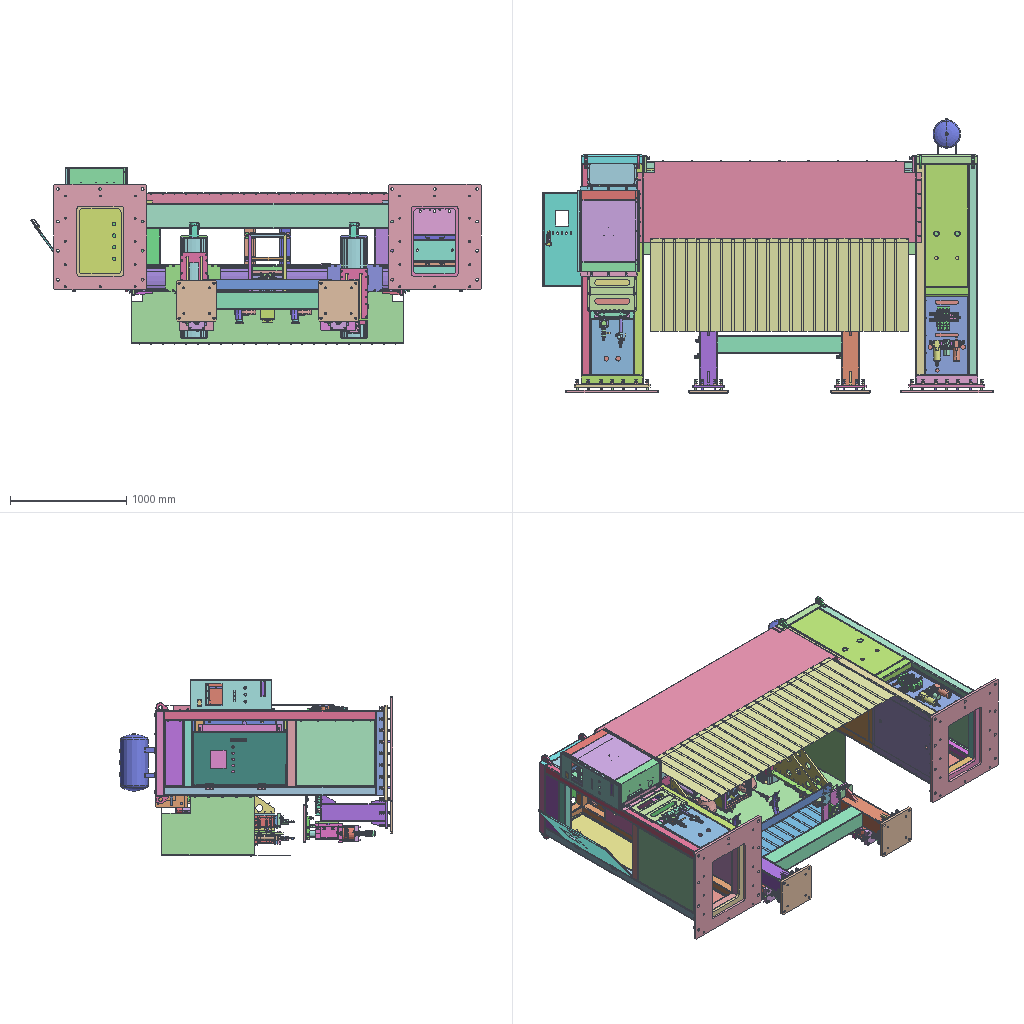Assembly | SolidWorks | 236 different items | 2045 placed | box 3873 x 2354 x 1514 mm
Parts list (item | name | quantity | parent item | size | volume | features):
1 | (subassembly) | x1 | - | - | 116635153 mm3 | -
2 | (subassembly) | x1 | in 1 | - | 39845939 mm3 | features ReferencePattern 84, LocalLPattern 9, CompositeCurve 3
3 | (subassembly) | x1 | in 1 | - | 39439593 mm3 | features ReferencePattern 3, CompositeCurve 2, LocalLPattern 1
4 | (subassembly) | x2 | in 1 | 203.047 x 914.102 x 280.36 mm | 3806317 mm3 | -
5 | (subassembly) | x2 | in 4 | 236 x 200 x 50 mm | 294173 mm3 | features HoleWzd 1
6 | (subassembly) | x2 | in 4 | 68 x 128 x 60 mm | 111810 mm3 | features HoleWzd 2
7 | (subassembly) | x1 | - | - | 32750415 mm3 | features ReferencePattern 33, LocalLPattern 4, CompositeCurve 3
8 | (subassembly) | x1 | in 26 | 248 x 227 x 99 mm | 1707610 mm3 | features AEMSimFeature 1
9 | (subassembly) | x2 | in 23 | 17.02 x 70 x 47.607 mm | 9149 mm3 | features AEMSimFeature 1
10 | (subassembly) | x1 | in 23 | 41.5 x 132 x 91.25 mm | 70272 mm3 | -
11 | (subassembly) | x2 | in 7 | 155 x 160 x 586.3 mm | 4938149 mm3 | features CompositeCurve 1
12 | (subassembly) | x2 | in 2, 3 | 305 x 58.518 x 57 mm | 304092 mm3 | features AEMSimFeature 1
13 | (subassembly) | x2 | in 14 | 152 x 98 x 38 mm | 442498 mm3 | -
14 | (subassembly) | x2 | in 7 | 152 x 98 x 38 mm | 442498 mm3 | -
15 | (subassembly) | x1 | in 25 | 91.219 x 83 x 33 mm | 40159 mm3 | -
16 | (subassembly) | x2 | in 2, 3 | 242 x 122 x 992.2 mm | 12646217 mm3 | features AEMSimFeature 1
17 | (subassembly) | x2 | in 2, 3 | 242 x 122 x 1042 mm | 13192618 mm3 | features AEMSimFeature 1
18 | (subassembly) | x2 | in 2, 3 | 35 x 30 x 30 mm | 22306 mm3 | features AEMSimFeature 1
19 | (subassembly) | x1 | in 26 | 209.8 x 130.6 x 274 mm | 1263291 mm3 | features ReferencePattern 6, LocalLPattern 1
20 | (subassembly) | x1 | in 25 | 68.642 x 53 x 59.392 mm | 27108 mm3 | -
21 | (subassembly) | x2 | in 4 | 110 x 140.16 x 248.72 mm | 144170 mm3 | -
22 | (subassembly) | x1 | in 25 | 57.569 x 74 x 99 mm | 152392 mm3 | -
23 | (subassembly) | x1 | - | - | 53716984 mm3 | features ReferencePattern 14, LocalLPattern 1
24 | (subassembly) | x1 | in 23 | 650 x 1995 x 900 mm | 30095229 mm3 | -
25 | (subassembly) | x1 | in 23 | 276.863 x 329.153 x 86.261 mm | 574652 mm3 | features CompositeCurve 2
26 | (subassembly) | x1 | - | - | 70550722 mm3 | features ReferencePattern 14, CompositeCurve 2, LocalLPattern 1
27 | (subassembly) | x1 | in 26 | 650 x 2000 x 900 mm | 28576602 mm3 | -
28 | - | x1 | in 26 | 306.443 x 240 x 500 mm | 20512353 mm3 | features ICE 5, HoleWzd 4, MirrorPattern 3, RefAxis 2, Extrusion 1, Revolution 1
29 | - | x1 | in 7 | 20.6 x 20 x 20 mm | 935.053 mm3 | features Revolution 1
30 | - | x4 | in 12 | 40 x 5.1 x 4.4 mm | 573.817 mm3 | features BaseBody 1
31 | - | x6 | in 16 | 13 x 15.5 x 39.5 mm | 3396 mm3 | features ICE 19, HoleWzd 5, Extrusion 1
32 | - | x6 | in 17 | 13 x 15.5 x 39.5 mm | 3396 mm3 | features ICE 19, HoleWzd 5, Extrusion 1
33 | - | x2 | in 16 | 220 x 113.5 x 15 mm | 261073 mm3 | features ICE 4, Chamfer 3, Extrusion 1, Fillet 1, HoleWzd 1
34 | - | x2 | in 17 | 220 x 113.5 x 15 mm | 261073 mm3 | features ICE 4, Chamfer 3, Extrusion 1, Fillet 1, HoleWzd 1
35 | - | x2 | in 16 | 188.037 x 25 x 1150 mm | 3794355 mm3 | features Extrusion 1, Fillet 1
36 | - | x2 | in 17 | 188.037 x 25 x 900 mm | 2969495 mm3 | features Extrusion 1, Fillet 1
37 | - | x2 | in 16 | 220 x 113.5 x 5 mm | 112175 mm3 | features Fillet 2, ICE 2, Chamfer 1, Extrusion 1
38 | - | x2 | in 17 | 220 x 113.5 x 5 mm | 112175 mm3 | features Fillet 2, ICE 2, Chamfer 1, Extrusion 1
39 | - | x2 | in 16 | 7 x 26.5 x 18 mm | 793.289 mm3 | features CornerTrim 1, FlatPattern 1, ICE 1, SMBaseFlange 1, SheetMetal 1
40 | - | x2 | in 16 | 220 x 67.5 x 1150 mm | 8709767 mm3 | features HoleWzd 3, ICE 3, Extrusion 1, Fillet 1, LPattern 1
41 | - | x2 | in 17 | 220 x 67.5 x 900 mm | 6810369 mm3 | features HoleWzd 3, ICE 3, Extrusion 1, Fillet 1, LPattern 1
42 | - | x2 | in 16 | 230 x 60 x 480 mm | 2333342 mm3 | features ICE 9, Fillet 3, HoleWzd 2, Chamfer 1, Cut 1, Extrusion 1, MirrorPattern 1
43 | - | x2 | in 17 | 230 x 60 x 480 mm | 2333342 mm3 | features ICE 9, Fillet 3, HoleWzd 2, Chamfer 1, Cut 1, Extrusion 1, MirrorPattern 1
44 | - | x2 | in 26 | 43.5 x 46 x 54 mm | 41092 mm3 | features BaseBody 1
45 | - | x4 | in 12 | 18 x 12.6 x 23 mm | 2035 mm3 | features BaseBody 1
46 | - | x4 | in 12 | 38 x 21 x 57 mm | 7816 mm3 | features BaseBody 1
47 | - | x2 | in 8 | 76 x 79.5 x 15.5 mm | 53255 mm3 | features BaseBody 1
48 | - | x1 | in 8 | 80 x 202.5 x 68 mm | 579205 mm3 | features BaseBody 1
49 | - | x1 | in 8 | 80 x 204.5 x 68 mm | 577118 mm3 | features BaseBody 1
50 | - | x2 | in 17 | 7 x 26.5 x 18 mm | 793.289 mm3 | features CornerTrim 1, FlatPattern 1, ICE 1, SMBaseFlange 1, SheetMetal 1
51 | - | x1 | in 8 | 80 x 140.5 x 83 mm | 444792 mm3 | features BaseBody 1
52 | - | x4 | in 7 | 70 x 25 x 14 mm | 23519 mm3 | features Extrusion 1, Fillet 1
53 | - | x2 | in 2 | 10 x 10 x 24 mm | 1497 mm3 | features Chamfer 3, Cut 2, Extrusion 1, RevCut 1
54 | - | x4 | - | 16 x 16 x 32 mm | 5349 mm3 | features Chamfer 3, Cut 2, Extrusion 1, RevCut 1
55 | - | x4 | in 2 | 6 x 6 x 22 mm | 513.442 mm3 | features Chamfer 3, Cut 2, Extrusion 1, RevCut 1
56 | - | x4 | in 2 | 8 x 8 x 30 mm | 1303 mm3 | features Chamfer 3, Cut 2, Extrusion 1, RevCut 1
57 | - | x78 | in 7, 23, 26 | 26.17 x 22.664 x 15.9 mm | 3864 mm3 | features Cut 2, Chamfer 1, Extrusion 1
58 | - | x4 | in 2 | 55.3 x 15.011 x 13 mm | 3268 mm3 | features RevCut 4, Chamfer 1, Extrusion 1, Fillet 1, LPattern 1, Revolution 1
59 | - | x4 | in 7 | 30.3 x 15.011 x 13 mm | 2011 mm3 | features RevCut 4, Chamfer 1, Extrusion 1, Fillet 1, LPattern 1, Revolution 1
60 | - | x50 | in 19 | 6.649 x 7.66 x 3.2 mm | 79.578 mm3 | features Cut 2, Chamfer 1, Extrusion 1
61 | - | x2 | in 25 | 26 x 31 x 10 mm | 2120 mm3 | features ICE 2, Revolution 1, Sweep 1
62 | - | x2 | in 26 | 12.482 x 14.38 x 6.8 mm | 562.42 mm3 | features Cut 2, Chamfer 1, Extrusion 1
63 | - | x4 | in 7 | 12.482 x 14.38 x 4 mm | 327.094 mm3 | features Cut 2, Chamfer 1, Extrusion 1
64 | - | x4 | in 2 | 30 x 16 x 16 mm | 3296 mm3 | features BlendCut 1, Cut 1, Fillet 1, LPattern 1, RevCut 1, Revolution 1
65 | - | x16 | in 4, 7 | 40 x 16 x 16 mm | 4081 mm3 | features BlendCut 1, Cut 1, Fillet 1, LPattern 1, RevCut 1, Revolution 1
66 | - | x6 | in 2 | 45 x 16 x 16 mm | 4474 mm3 | features BlendCut 1, Cut 1, Fillet 1, LPattern 1, RevCut 1, Revolution 1
67 | - | x32 | in 7, 23, 26 | 116 x 24 x 24 mm | 25974 mm3 | features BlendCut 1, Cut 1, Fillet 1, LPattern 1, RevCut 1, Revolution 1
68 | - | x20 | - | 56 x 24 x 24 mm | 13910 mm3 | features BlendCut 1, Cut 1, Fillet 1, LPattern 1, RevCut 1, Revolution 1
69 | - | x12 | in 7 | 71 x 24 x 24 mm | 16926 mm3 | features BlendCut 1, Cut 1, Fillet 1, LPattern 1, RevCut 1, Revolution 1
70 | - | x44 | in 7, 23, 26 | 96 x 24 x 24 mm | 21953 mm3 | features BlendCut 1, Cut 1, Fillet 1, LPattern 1, RevCut 1, Revolution 1
71 | - | x28 | in 16 | 9 x 5.5 x 5.5 mm | 106.317 mm3 | features BlendCut 1, Cut 1, Fillet 1, RevCut 1, Revolution 1
72 | - | x8 | in 2, 25 | 16.166 x 31 x 14 mm | 2228 mm3 | features ICE 3, Chamfer 1, Revolution 1
73 | - | x28 | in 17 | 9 x 5.5 x 5.5 mm | 106.317 mm3 | features BlendCut 1, Cut 1, Fillet 1, RevCut 1, Revolution 1
74 | - | x46 | - | 16 x 7 x 7 mm | 288.227 mm3 | features BlendCut 1, Cut 1, Fillet 1, LPattern 1, RevCut 1, Revolution 1
75 | - | x4 | in 19 | 44 x 7 x 7 mm | 640.086 mm3 | features BlendCut 1, Cut 1, Fillet 1, LPattern 1, RevCut 1, Revolution 1
76 | - | x222 | in 23, 26 | 12 x 7 x 7 mm | 237.962 mm3 | features BlendCut 1, Cut 1, Fillet 1, LPattern 1, RevCut 1, Revolution 1
77 | - | x38 | - | 16 x 10 x 10 mm | 686.638 mm3 | features BlendCut 1, Cut 1, Fillet 1, LPattern 1, RevCut 1, Revolution 1
78 | - | x8 | in 7 | 26 x 10 x 10 mm | 969.381 mm3 | features BlendCut 1, Cut 1, Fillet 1, LPattern 1, RevCut 1, Revolution 1
79 | - | x4 | in 7 | 36 x 10 x 10 mm | 1252 mm3 | features BlendCut 1, Cut 1, Fillet 1, LPattern 1, RevCut 1, Revolution 1
80 | - | x4 | in 7 | 46 x 10 x 10 mm | 1535 mm3 | features BlendCut 1, Cut 1, Fillet 1, LPattern 1, RevCut 1, Revolution 1
81 | - | x10 | in 23 | 24 x 13 x 13 mm | 1736 mm3 | features BlendCut 1, Cut 1, Fillet 1, LPattern 1, RevCut 1, Revolution 1
82 | - | x28 | in 7 | 28 x 13 x 13 mm | 1937 mm3 | features BlendCut 1, Cut 1, Fillet 1, LPattern 1, RevCut 1, Revolution 1
83 | - | x1 | in 19 | 75 x 28 x 192 mm | 234020 mm3 | features BaseBody 1
84 | - | x49 | in 2, 26 | 33 x 13 x 13 mm | 2189 mm3 | features BlendCut 1, Cut 1, Fillet 1, LPattern 1, RevCut 1, Revolution 1
85 | - | x28 | in 2 | 38 x 13 x 13 mm | 2440 mm3 | features BlendCut 1, Cut 1, Fillet 1, LPattern 1, RevCut 1, Revolution 1
86 | - | x28 | in 2, 23 | 48 x 13 x 13 mm | 2943 mm3 | features BlendCut 1, Cut 1, Fillet 1, LPattern 1, RevCut 1, Revolution 1
87 | - | x12 | in 23 | 10 x 8.96 x 8.96 mm | 171.604 mm3 | features RevCut 2, Revolution 2, Cut 1, LPattern 1, RefAxis 1
88 | - | x4 | in 4 | 10 x 8 x 8 mm | 368.793 mm3 | features RevCut 2, Cut 1, LPattern 1, Revolution 1
89 | - | x18 | in 2, 4 | 15.372 x 15.344 x 2.6 mm | 261.313 mm3 | features Extrusion 1
90 | - | x32 | in 7 | 24.356 x 24.313 x 4.1 mm | 1031 mm3 | features Extrusion 1
91 | - | x272 | in 19, 23, 26 | 6.287 x 6.275 x 1.1 mm | 18.963 mm3 | features Extrusion 1
92 | - | x46 | in 7 | 9.282 x 9.265 x 1.6 mm | 59.463 mm3 | features Extrusion 1
93 | - | x30 | in 2, 23 | 12.277 x 12.254 x 2.1 mm | 135.755 mm3 | features Extrusion 1
94 | - | x4 | in 19 | 27 x 69.3 x 209.8 mm | 222441 mm3 | features BaseBody 1
95 | - | x8 | in 4 | 20 x 2 x 20 mm | 438.252 mm3 | features Revolution 1
96 | - | x32 | in 7 | 30 x 3 x 30 mm | 1399 mm3 | features Revolution 1
97 | - | x276 | in 19, 23, 26 | 9 x 0.8 x 9 mm | 38.17 mm3 | features Revolution 1
98 | - | x46 | in 7 | 12 x 1.6 x 12 mm | 127.863 mm3 | features Revolution 1
99 | - | x26 | in 23 | 16 x 1.6 x 16 mm | 219.911 mm3 | features Revolution 1
100 | - | x4 | in 2 | 20 x 2 x 20 mm | 455.138 mm3 | features Revolution 1
101 | - | x2 | in 9 | 8 x 70 x 29 mm | 3838 mm3 | features BaseBody 1
102 | - | x2 | in 9 | 8 x 70 x 29 mm | 4432 mm3 | features BaseBody 1
103 | - | x2 | in 9 | 4 x 70 x 4 mm | 879.661 mm3 | features BaseBody 1
104 | - | x1 | in 23 | - | 3525284 mm3 | features BaseBody 46
105 | - | x1 | in 25 | 33.486 x 29 x 29 mm | 7069 mm3 | features ICE 3, Chamfer 1, Extrusion 1, HoleWzd 1
106 | - | x1 | in 1 | 128 x 196 x 428.2 mm | 1860120 mm3 | features BaseBody 23
107 | - | x2 | in 19 | 64.8 x 11 x 27.5 mm | 5589 mm3 | features BaseBody 1
108 | - | x2 | in 19 | 26 x 68 x 26.213 mm | 26023 mm3 | features BaseBody 1
109 | - | x1 | in 26 | 19.63 x 32.5 x 17 mm | 4456 mm3 | features BaseBody 1
110 | - | x2 | in 19 | 35.315 x 37 x 18 mm | 6710 mm3 | features BaseBody 1
111 | - | x2 | in 26 | 37.624 x 41.5 x 21 mm | 10136 mm3 | features BaseBody 1
112 | - | x3 | in 19 | 32.815 x 34 x 17 mm | 6015 mm3 | features BaseBody 1
113 | - | x1 | in 19 | 35.315 x 63.5 x 18 mm | 9000 mm3 | features BaseBody 1
114 | - | x3 | in 19 | 32.815 x 55.5 x 17 mm | 7231 mm3 | features BaseBody 1
115 | - | x4 | in 7 | 49.5 x 58.5 x 28 mm | 24100 mm3 | features BaseBody 1
116 | - | x2 | in 11 | 125 x 125 x 5.7 mm | 25182 mm3 | features BaseBody 1
117 | - | x4 | in 7 | 33.5 x 41.5 x 15 mm | 5375 mm3 | features BaseBody 1
118 | - | x2 | in 2 | 37.5 x 47.5 x 18 mm | 8206 mm3 | features BaseBody 1
119 | - | x4 | in 2 | 40.75 x 52.5 x 22.5 mm | 13948 mm3 | features BaseBody 1
120 | - | x8 | in 12 | 22 x 10 x 10 mm | 853.724 mm3 | features BaseBody 1
121 | - | x2 | in 12 | 7 x 19.63 x 17 mm | 1102 mm3 | features BaseBody 1
122 | - | x2 | in 12 | 232.5 x 39.5 x 39.5 mm | 68995 mm3 | features BaseBody 1
123 | - | x2 | in 12 | 233 x 50 x 50 mm | 209735 mm3 | features BaseBody 1
124 | - | x2 | in 13 | 136 x 38 x 98 mm | 311223 mm3 | features BaseBody 1
125 | - | x2 | in 13 | 143.5 x 36 x 96 mm | 131275 mm3 | features BaseBody 1
126 | - | x2 | in 11 | 25 x 25 x 150 mm | 71513 mm3 | features BaseBody 1
127 | - | x6 | in 16 | 25 x 17 x 16 mm | 1093 mm3 | features EdgeFlange 1, Fillet 1, FlatPattern 1, HoleWzd 1, ICE 1, MirrorPattern 1, SMBaseFlange 1, SheetMetal 1
128 | - | x8 | in 11 | 14.038 x 16 x 170 mm | 19424 mm3 | features BaseBody 1
129 | - | x2 | in 11 | 229 x 32 x 32 mm | 152492 mm3 | features BaseBody 1
130 | - | x2 | in 11 | 50 x 50 x 5 mm | 5541 mm3 | features BaseBody 1
131 | - | x2 | in 11 | 44.103 x 44.731 x 12 mm | 9622 mm3 | features BaseBody 1
132 | - | x2 | in 16 | 80.44 x 89.02 x 162.2 mm | 690477 mm3 | features BaseBody 1
133 | - | x2 | in 17 | 80.44 x 89.02 x 162.2 mm | 690477 mm3 | features BaseBody 1
134 | - | x2 | in 21 | 94 x 8 x 103 mm | 10565 mm3 | features ICE 1, Sweep 1
135 | - | x4 | in 21 | 15.011 x 13 x 7.9 mm | 844.03 mm3 | features Chamfer 2, RevCut 2, Extrusion 1, ICE 1, LPattern 1
136 | - | x4 | in 21 | 15.011 x 13 x 4 mm | 430.713 mm3 | features RevCut 2, Chamfer 1, Extrusion 1, LPattern 1
137 | - | x2 | in 4 | 20 x 15.24 x 15.24 mm | 1317 mm3 | features RevCut 3, Chamfer 1, Cut 1, Fillet 1, LPattern 1, Revolution 1
138 | - | x2 | in 18 | 28 x 30 x 30 mm | 9162 mm3 | features BaseBody 1
139 | - | x6 | in 17 | 25 x 17 x 16 mm | 1093 mm3 | features EdgeFlange 1, Fillet 1, FlatPattern 1, HoleWzd 1, ICE 1, MirrorPattern 1, SMBaseFlange 1, SheetMetal 1
140 | - | x1 | in 27 | 650 x 2000 x 880 mm | 28196687 mm3 | features HoleWzd 24, WeldCornerFeat 14, ICE 8, WeldMemberFeat 4, Chamfer 2, Fillet 2, 3DProfileFeature 1, WeldmentFeature 1
141 | - | x4 | in 24 | 70 x 110 x 20 mm | 94979 mm3 | features Fillet 3, Extrusion 1, ICE 1
142 | - | x4 | in 27 | 70 x 110 x 20 mm | 94979 mm3 | features Fillet 3, Extrusion 1, ICE 1
143 | - | x1 | in 24 | 650 x 1995 x 880 mm | 29715314 mm3 | features HoleWzd 25, WeldCornerFeat 15, ICE 11, Chamfer 8, WeldMemberFeat 3, Fillet 2, LPattern 2, MoveFace 2, 3DProfileFeature 1, WeldmentFeature 1
144 | - | x4 | in 21 | 16 x 16 x 1.6 mm | 233.031 mm3 | features Extrusion 1
145 | - | x2 | in 4 | 130 x 538 x 180 mm | 2549222 mm3 | features BaseBody 3
146 | - | x1 | in 25 | 27 x 27 x 154 mm | 47629 mm3 | features ICE 2, Chamfer 1, Extrusion 1, MirrorPattern 1
147 | - | x1 | in 25 | 240 x 40 x 30 mm | 239495 mm3 | features HoleWzd 6, MirrorPattern 2, Extrusion 1
148 | - | x2 | in 25 | 31.177 x 58 x 27 mm | 12376 mm3 | features ICE 4, Chamfer 2, Revolution 1
149 | - | x2 | in 11 | 125 x 125 x 8.6 mm | 37994 mm3 | features BaseBody 1
150 | - | x2 | in 2, 3 | 100 x 577.1 x 113 mm | 2394119 mm3 | features BaseBody 23, ICE 1
151 | - | x2 | in 21 | 110 x 51.16 x 248.72 mm | 85285 mm3 | features Chamfer 4, Fillet 2, HoleWzd 2, ICE 2, BossThin 1, Revolution 1, Shell 1
152 | - | x2 | in 21 | 110 x 15 x 125 mm | 45305 mm3 | features Chamfer 4, Fillet 2, ICE 2, ExtruThin 1, HoleWzd 1
153 | - | x3 | in 19 | 19.63 x 16 x 17 mm | 3623 mm3 | features BaseBody 1
154 | - | x1 | in 22 | 41.569 x 55 x 99 mm | 62530 mm3 | features ICE 5, HoleWzd 2, Extrusion 1, MirrorPattern 1
155 | - | x2 | in 22 | 74 x 74 x 13 mm | 39480 mm3 | features ICE 2, 3DProfileFeature 1, Chamfer 1, Extrusion 1, HoleWzd 1
156 | - | x1 | in 22 | 54.5 x 54.5 x 4 mm | 9331 mm3 | features Extrusion 1
157 | - | x2 | in 11 | 130 x 130 x 30 mm | 407669 mm3 | features BaseBody 1
158 | - | x1 | in 22 | 55 x 55 x 2 mm | 1571 mm3 | features Extrusion 1
159 | - | x1 | in 25 | 31.177 x 27 x 27 mm | 5569 mm3 | features ICE 3, Extrusion 1, SweepThread 1
160 | - | x1 | in 25 | 31.177 x 27 x 43 mm | 12851 mm3 | features ICE 2, Chamfer 1, Extrusion 1, MirrorPattern 1
161 | - | x1 | in 15 | 30 x 30 x 15.2 mm | 4101 mm3 | features ICE 3, Extrusion 1
162 | - | x1 | in 20 | 33 x 53.25 x 53 mm | 25680 mm3 | features ICE 10, HoleWzd 2, 3DProfileFeature 1, Extrusion 1, Fillet 1
163 | - | x1 | in 15 | 33 x 81.096 x 83 mm | 34631 mm3 | features ICE 13, HoleWzd 3, 3DProfileFeature 2, Extrusion 1, Fillet 1, Sweep 1
164 | - | x2 | in 15, 20 | 62.879 x 15.737 x 21.142 mm | 1428 mm3 | features EdgeFlange 4, Fillet 2, ICE 2, FlatPattern 1, SMBaseFlange 1, SheetMetal 1
165 | - | x2 | in 7 | 140 x 25 x 36 mm | 123238 mm3 | features Chamfer 1, Extrusion 1, HoleWzd 1
166 | - | x1 | - | 2461 x 800 x 510 mm | 7657970 mm3 | features ICE 4, EdgeFlange 2, LPattern 2, FlatPattern 1, SMBaseFlange 1, SheetMetal 1
167 | - | x1 | - | 2441 x 700 x 150 mm | 4096211 mm3 | features ICE 4, EdgeFlange 3, LPattern 2, FlatPattern 1, SMBaseFlange 1, SheetMetal 1
168 | - | x2 | in 11 | 160 x 155 x 246 mm | 1955692 mm3 | features ICE 2, BaseBody 1
169 | - | x22 | - | 120 x 350 x 2 mm | 83936 mm3 | features Extrusion 1, ICE 1
170 | - | x22 | - | 120 x 800 x 2 mm | 191936 mm3 | features Extrusion 1, ICE 1
171 | - | x1 | in 23 | 420 x 180 x 2 mm | 150541 mm3 | features RefAxis 2, Extrusion 1, Fillet 1, HoleWzd 1, ICE 1
172 | - | x2 | in 23, 26 | 1048 x 368 x 25 mm | 891323 mm3 | features EdgeFlange 1, FlatPattern 1, ICE 1, SMBaseFlange 1, SheetMetal 1
173 | - | x2 | in 23, 26 | 568 x 158 x 25 mm | 241019 mm3 | features EdgeFlange 1, FlatPattern 1, ICE 1, SMBaseFlange 1, SheetMetal 1
174 | - | x2 | in 23, 26 | 680 x 568 x 25 mm | 878615 mm3 | features EdgeFlange 1, FlatPattern 1, ICE 1, SMBaseFlange 1, SheetMetal 1
175 | - | x2 | in 23, 26 | 680 x 368 x 25 mm | 589246 mm3 | features EdgeFlange 1, FlatPattern 1, ICE 1, SMBaseFlange 1, SheetMetal 1
176 | - | x1 | in 23 | 700 x 780 x 2 mm | 1090782 mm3 | features Extrusion 1, ICE 1
177 | - | x1 | in 23 | 420 x 300 x 2 mm | 193243 mm3 | features ICE 2, Extrusion 1, Fillet 1, HoleWzd 1, MirrorPattern 1
178 | - | x1 | in 23 | 500 x 714 x 50 mm | 1369290 mm3 | features EdgeFlange 2, FlatPattern 1, ICE 1, SMBaseFlange 1, SheetMetal 1
179 | - | x2 | in 11 | 24 x 124 x 124 mm | 184707 mm3 | features BaseBody 1
180 | - | x1 | in 23 | 566 x 15 x 806 mm | 720879 mm3 | features ICE 3, EdgeFlange 2, Cut 1, FlatPattern 1, LPattern 1, SMBaseFlange 1, SheetMetal 1
181 | - | x2 | in 23 | 47 x 25 x 20 mm | 4405 mm3 | features EdgeFlange 2, Fillet 1, FlatPattern 1, ICE 1, SMBaseFlange 1, SheetMetal 1
182 | - | x1 | in 23 | 40 x 35 x 50 mm | 8331 mm3 | features EdgeFlange 3, RefAxis 3, Fillet 2, ICE 2, FlatPattern 1, SMBaseFlange 1, SheetMetal 1
183 | - | x1 | in 23 | 700 x 500 x 2 mm | 691794 mm3 | features Extrusion 1, HoleWzd 1, ICE 1
184 | - | x2 | in 23, 26 | 800 x 905 x 20 mm | 9564492 mm3 | features HoleWzd 2, ICE 2, Chamfer 1, Extrusion 1, Fillet 1
185 | - | x1 | in 23 | 479 x 368 x 25 mm | 418826 mm3 | features ICE 2, EdgeFlange 1, FlatPattern 1, SMBaseFlange 1, SheetMetal 1
186 | - | x1 | in 23 | 15 x 650 x 420 mm | 545219 mm3 | features ICE 4, EdgeFlange 1, FlatPattern 1, HoleWzd 1, SMBaseFlange 1, SheetMetal 1
187 | - | x1 | in 23 | 700 x 900 x 2 mm | 1238676 mm3 | features ICE 2, Extrusion 1
188 | - | x1 | in 26 | 810 x 570 x 25 mm | 1040756 mm3 | features EdgeFlange 1, FlatPattern 1, ICE 1, SMBaseFlange 1, SheetMetal 1
189 | - | x1 | in 26 | 680 x 370 x 25 mm | 562100 mm3 | features ICE 4, Cut 1, EdgeFlange 1, FlatPattern 1, HoleWzd 1, SMBaseFlange 1, SheetMetal 1
190 | - | x2 | in 11 | 135 x 135 x 104.3 mm | 212984 mm3 | features BaseBody 1
191 | - | x1 | in 26 | 1050 x 370 x 25 mm | 888515 mm3 | features ICE 2, Cut 1, EdgeFlange 1, FlatPattern 1, LPattern 1, SMBaseFlange 1, SheetMetal 1
192 | - | x1 | in 26 | 295 x 500 x 2 mm | 292699 mm3 | features Extrusion 1, HoleWzd 1, ICE 1
193 | - | x1 | in 26 | 355 x 500 x 2 mm | 307692 mm3 | features ICE 2, Extrusion 1, Fillet 1, HoleWzd 1
194 | - | x1 | in 26 | 700 x 900 x 2 mm | 1258782 mm3 | features Extrusion 1, ICE 1
195 | - | x1 | in 26 | 700 x 760 x 2 mm | 1059954 mm3 | features Cut 1, Extrusion 1, ICE 1
196 | - | x1 | in 1 | 2320 x 250 x 830 mm | 26047489 mm3 | features ICE 14, HoleWzd 6, WeldMemberFeat 3, Chamfer 2, 3DProfileFeature 1, Cut 1, WeldCornerFeat 1, WeldmentFeature 1
197 | - | x1 | in 1 | 523 x 375 x 640 mm | 1667392 mm3 | features WeldCornerFeat 4, HoleWzd 2, ICE 2, 3DProfileFeature 1, WeldMemberFeat 1, WeldmentFeature 1
198 | - | x2 | in 1 | 260 x 45 x 50 mm | 79882 mm3 | features ICE 2, Chamfer 1, FlatPattern 1, SMBaseFlange 1, SheetMetal 1
199 | - | x1 | in 2 | 480 x 880 x 16 mm | 3786407 mm3 | features HoleWzd 4, Chamfer 1, Extrusion 1, Fillet 1, ICE 1
200 | - | x2 | in 2, 3 | 480 x 235 x 16 mm | 1317910 mm3 | features HoleWzd 5, ICE 3, Chamfer 1, Extrusion 1, Fillet 1, LPattern 1
201 | - | x2 | in 11 | 50 x 50 x 75 mm | 76101 mm3 | features BaseBody 1
202 | - | x1 | in 2 | 16 x 550 x 235 mm | 1648146 mm3 | features HoleWzd 5, ICE 4, Chamfer 1, Extrusion 1, Fillet 1, LPattern 1
203 | - | x4 | in 2, 3 | 385 x 550 x 16 mm | 1761626 mm3 | features HoleWzd 2, LPattern 2, Extrusion 1, ICE 1
204 | - | x2 | in 2, 3 | 100 x 80 x 2 mm | 14938 mm3 | features Extrusion 1, ICE 1
205 | - | x1 | in 2 | 120 x 80 x 95 mm | 309106 mm3 | features HoleWzd 5, ICE 4, Chamfer 1, Extrusion 1, Fillet 1, RevCut 1
206 | - | x2 | in 2, 3 | 50 x 18 x 18 mm | 5917 mm3 | features ICE 1, Revolution 1
207 | - | x2 | in 2, 3 | 16 x 25 x 16 mm | 2776 mm3 | features Chamfer 1, Extrusion 1, RevCut 1
208 | - | x2 | in 2, 3 | 60 x 345 x 16 mm | 288953 mm3 | features RefAxis 4, HoleWzd 3, ICE 2, Chamfer 1, Extrusion 1
209 | - | x8 | in 2, 3 | 12.4 x 18 x 18 mm | 530.163 mm3 | features Revolution 1
210 | - | x1 | in 3 | 480 x 880 x 16 mm | 3786407 mm3 | features HoleWzd 4, Chamfer 2, Extrusion 1, Fillet 1, ICE 1
211 | - | x1 | in 3 | 16 x 550 x 235 mm | 1648646 mm3 | features HoleWzd 5, ICE 4, Chamfer 1, Extrusion 1, Fillet 1, LPattern 1
212 | - | x2 | in 11 | 145 x 145 x 40 mm | 721249 mm3 | features BaseBody 1, Cut 1
213 | - | x1 | in 3 | 110 x 80 x 95 mm | 289106 mm3 | features HoleWzd 5, ICE 4, Chamfer 1, Extrusion 1, Fillet 1, RevCut 1
214 | - | x2 | in 5 | 50 x 50 x 200 mm | 131874 mm3 | features Extrusion 1, ICE 1, WeldmentFeature 1
215 | - | x2 | in 5 | 20 x 120 x 5 mm | 9312 mm3 | features Chamfer 1, Extrusion 1
216 | - | x2 | in 5 | 50 x 50 x 200 mm | 141372 mm3 | features Extrusion 1
217 | - | x2 | in 5 | 50 x 50 x 6 mm | 11781 mm3 | features Extrusion 1
218 | - | x2 | in 4 | 100 x 100 x 366 mm | 643224 mm3 | features ICE 3, HoleWzd 2, Chamfer 1, Extrusion 1
219 | - | x2 | in 6 | 68 x 68 x 60 mm | 90478 mm3 | features Extrusion 1, WeldmentFeature 1
220 | - | x2 | in 6 | 60 x 60 x 10 mm | 21914 mm3 | features Chamfer 2, Extrusion 1
221 | - | x2 | in 4 | 50 x 50 x 5 mm | 9077 mm3 | features Chamfer 1, Extrusion 1, HoleWzd 1
222 | - | x2 | in 4 | 50 x 50 x 5 mm | 3534 mm3 | features Extrusion 1
223 | - | x2 | in 11 | 379.7 x 60 x 60 mm | 998065 mm3 | features BaseBody 1
224 | - | x2 | in 4 | 70 x 70 x 8 mm | 29565 mm3 | features Chamfer 1, Extrusion 1, HoleWzd 1
225 | - | x1 | in 7 | 1490 x 295 x 618 mm | 10128705 mm3 | features ICE 6, HoleWzd 5, Chamfer 4, 3DProfileFeature 1, MirrorPattern 1, WeldMemberFeat 1, WeldmentFeature 1
226 | - | x1 | in 7 | 1100 x 80 x 10 mm | 856189 mm3 | features ICE 2, Extrusion 1, HoleWzd 1
227 | - | x2 | in 7 | 130 x 130 x 4 mm | 65444 mm3 | features Chamfer 1, Extrusion 1, HoleWzd 1
228 | - | x1 | in 7 | 300 x 320 x 20 mm | 1873413 mm3 | features HoleWzd 2, Chamfer 1, Extrusion 1, ICE 1
229 | - | x2 | in 7 | 350 x 350 x 20 mm | 2411003 mm3 | features HoleWzd 2, Chamfer 1, Extrusion 1
230 | - | x2 | in 7 | 180 x 45 x 20 mm | 111535 mm3 | features HoleWzd 2, Chamfer 1, Extrusion 1, Fillet 1, ICE 1
231 | - | x2 | in 7 | 180 x 45 x 20 mm | 111535 mm3 | features HoleWzd 2, Chamfer 1, Extrusion 1, Fillet 1, ICE 1
232 | - | x1 | in 7 | 300 x 320 x 20 mm | 1873413 mm3 | features HoleWzd 2, Chamfer 1, Extrusion 1, ICE 1
233 | - | x2 | in 7 | 200 x 90 x 10 mm | 176073 mm3 | features HoleWzd 2, ICE 2, Extrusion 1
234 | - | x2 | in 18 | 25 x 30 x 30 mm | 13143 mm3 | features BaseBody 1
235 | SR20008JN (subassembly) | x1 | - | - | - | -
236 | Nameplate | x1 | - | - | - | -
Mates (type | each side: item.copy, entity, surface, feature), first 379 of 3009 lines:
In the top assembly
Coincident | 23.1 plane | assembly plane | 3 times
Coincident | 23.1 plane | 26.1 plane
Coincident | 143.1 face plane Cut-Extrude 2 | 196.1 face plane Boss-Extrude 4 | 2 times
Coincident | 140.1 face plane Cut-Extrude 2 | 196.1 face plane Boss-Extrude 1 | 2 times
Coincident | 184.1 face plane Boss-Extrude 1 | 229.1 face plane Boss-Extrude 1
Width | 168.1 face plane Import 1 | 168.2 face plane Import 1 | 196.1 face plane Boss-Extrude 1 | 196.1 face plane Boss-Extrude 4
DistanceDim | 225.1 face plane Boss-Extrude 8 | 140.1 face plane Square Tube 80×80×4.0(2)
Coincident | 140.1 face plane Square Tube 80×80×4.0(2) | 166.1 face plane Edge-Flange 2
Coincident | 196.1 face plane Rect Tube 220×140×5(1) | 166.1 face plane Edge-Flange 1
Width | 166.1 face plane Edge-Flange 1 | 166.1 face plane Edge-Flange 1 | 196.1 face plane Boss-Extrude 1 | 196.1 face plane Boss-Extrude 4
Width | 167.1 face plane Edge-Flange 1 | 167.1 face plane Edge-Flange 1 | 196.1 face plane Boss-Extrude 4 | 196.1 face plane Boss-Extrude 1
Coincident | 143.1 face plane Square Tube 80×80×4.0(2) | 167.1 face plane Edge-Flange 2
Coincident | 196.1 face plane Rect Tube 220×140×5(1) | 167.1 face plane Edge-Flange 3
Coincident | 166.1 face plane Base-Flange 1 | 169.1 face plane Boss-Extrude 1
Concentric | 166.1 face cylinder Cut-Extrude 6 | 169.1 face cylinder Cut-Extrude 1
Concentric | 166.1 face cylinder LPattern 2 | 169.1 face cylinder Cut-Extrude 1
Coincident | 167.1 face plane Base-Flange 1 | 170.1 face plane Boss-Extrude 1
Concentric | 167.1 face cylinder Cut-Extrude 4 | 170.1 face cylinder Cut-Extrude 1
Concentric | 167.1 face cylinder LPattern 2 | 170.1 face cylinder Cut-Extrude 1
Concentric | 140.1 face cylinder M16 Tapped Hole 2 | 196.1 face cylinder Ø16.5 (16.5) DiameterHole 1
Concentric | 68.1 face cylinder Base-Revolve | 96.1 face cylinder Base-Revolve
Coincident | 68.1 face plane Base-Revolve | 90.1 face plane Extrude 1
Concentric | 96.1 face cylinder Base-Revolve | 90.1 face cylinder Extrude 1
Coincident | 96.1 face plane Base-Revolve | 90.1 face plane Extrude 1
Concentric | 196.1 face cylinder Ø16.5 (16.5) DiameterHole 1 | 68.1 face cylinder Base-Revolve
Coincident | 196.1 face plane Boss-Extrude 1 | 96.1 face plane Base-Revolve
Concentric | 68.2 face cylinder Base-Revolve | 96.2 face cylinder Base-Revolve
Coincident | 68.2 face plane Base-Revolve | 90.2 face plane Extrude 1
Concentric | 96.2 face cylinder Base-Revolve | 90.2 face cylinder Extrude 1
Coincident | 96.2 face plane Base-Revolve | 90.2 face plane Extrude 1
Concentric | 196.1 face cylinder Ø16.5 (16.5) DiameterHole 1 | 68.2 face cylinder Base-Revolve
Coincident | 196.1 face plane Boss-Extrude 1 | 96.2 face plane Base-Revolve
Concentric | 68.3 face cylinder Base-Revolve | 96.3 face cylinder Base-Revolve
Coincident | 68.3 face plane Base-Revolve | 90.3 face plane Extrude 1
Concentric | 96.3 face cylinder Base-Revolve | 90.3 face cylinder Extrude 1
Coincident | 96.3 face plane Base-Revolve | 90.3 face plane Extrude 1
Concentric | 196.1 face cylinder Ø16.5 (16.5) DiameterHole 1 | 68.3 face cylinder Base-Revolve
Coincident | 196.1 face plane Boss-Extrude 1 | 96.3 face plane Base-Revolve
Concentric | 68.4 face cylinder Base-Revolve | 96.4 face cylinder Base-Revolve
Coincident | 68.4 face plane Base-Revolve | 90.4 face plane Extrude 1
Concentric | 96.4 face cylinder Base-Revolve | 90.4 face cylinder Extrude 1
Coincident | 96.4 face plane Base-Revolve | 90.4 face plane Extrude 1
Concentric | 196.1 face cylinder Ø16.5 (16.5) DiameterHole 1 | 68.4 face cylinder Base-Revolve
Coincident | 196.1 face plane Boss-Extrude 1 | 96.4 face plane Base-Revolve
Concentric | 68.5 face cylinder Base-Revolve | 96.5 face cylinder Base-Revolve
Coincident | 68.5 face plane Base-Revolve | 90.5 face plane Extrude 1
Concentric | 96.5 face cylinder Base-Revolve | 90.5 face cylinder Extrude 1
Coincident | 96.5 face plane Base-Revolve | 90.5 face plane Extrude 1
Concentric | 196.1 face cylinder Ø16.5 (16.5) DiameterHole 1 | 68.5 face cylinder Base-Revolve
Coincident | 196.1 face plane Boss-Extrude 1 | 96.5 face plane Base-Revolve
Concentric | 68.6 face cylinder Base-Revolve | 96.6 face cylinder Base-Revolve
Coincident | 68.6 face plane Base-Revolve | 90.6 face plane Extrude 1
Concentric | 96.6 face cylinder Base-Revolve | 90.6 face cylinder Extrude 1
Coincident | 96.6 face plane Base-Revolve | 90.6 face plane Extrude 1
Concentric | 196.1 face cylinder Ø16.5 (16.5) DiameterHole 1 | 68.6 face cylinder Base-Revolve
Coincident | 196.1 face plane Boss-Extrude 1 | 96.6 face plane Base-Revolve
Concentric | 68.7 face cylinder Base-Revolve | 96.7 face cylinder Base-Revolve
Coincident | 68.7 face plane Base-Revolve | 90.7 face plane Extrude 1
Concentric | 96.7 face cylinder Base-Revolve | 90.7 face cylinder Extrude 1
Coincident | 96.7 face plane Base-Revolve | 90.7 face plane Extrude 1
Concentric | 196.1 face cylinder Ø16.5 (16.5) DiameterHole 1 | 68.7 face cylinder Base-Revolve
Coincident | 196.1 face plane Boss-Extrude 1 | 96.7 face plane Base-Revolve
Concentric | 68.8 face cylinder Base-Revolve | 96.8 face cylinder Base-Revolve
Coincident | 68.8 face plane Base-Revolve | 90.8 face plane Extrude 1
Concentric | 96.8 face cylinder Base-Revolve | 90.8 face cylinder Extrude 1
Coincident | 96.8 face plane Base-Revolve | 90.8 face plane Extrude 1
Concentric | 196.1 face cylinder Ø16.5 (16.5) DiameterHole 1 | 68.8 face cylinder Base-Revolve
Coincident | 196.1 face plane Boss-Extrude 1 | 96.8 face plane Base-Revolve
Concentric | 68.9 face cylinder Base-Revolve | 96.9 face cylinder Base-Revolve
Coincident | 68.9 face plane Base-Revolve | 90.9 face plane Extrude 1
Concentric | 96.9 face cylinder Base-Revolve | 90.9 face cylinder Extrude 1
Coincident | 96.9 face plane Base-Revolve | 90.9 face plane Extrude 1
Concentric | 196.1 face cylinder Ø16.5 (16.5) DiameterHole 1 | 68.9 face cylinder Base-Revolve
Coincident | 196.1 face plane Boss-Extrude 1 | 96.9 face plane Base-Revolve
Concentric | 68.10 face cylinder Base-Revolve | 96.10 face cylinder Base-Revolve
Coincident | 68.10 face plane Base-Revolve | 90.10 face plane Extrude 1
Concentric | 96.10 face cylinder Base-Revolve | 90.10 face cylinder Extrude 1
Coincident | 96.10 face plane Base-Revolve | 90.10 face plane Extrude 1
Concentric | 196.1 edge | 68.10 face cylinder Base-Revolve
Coincident | 196.1 face plane Boss-Extrude 1 | 96.10 face plane Base-Revolve
Concentric | 68.11 face cylinder Base-Revolve | 96.11 face cylinder Base-Revolve
Coincident | 68.11 face plane Base-Revolve | 90.11 face plane Extrude 1
Concentric | 96.11 face cylinder Base-Revolve | 90.11 face cylinder Extrude 1
Coincident | 96.11 face plane Base-Revolve | 90.11 face plane Extrude 1
Concentric | 196.1 face cylinder Ø16.5 (16.5) DiameterHole 1 | 68.11 face cylinder Base-Revolve
Coincident | 196.1 face plane Boss-Extrude 4 | 96.11 face plane Base-Revolve
Concentric | 68.12 face cylinder Base-Revolve | 96.12 face cylinder Base-Revolve
Coincident | 68.12 face plane Base-Revolve | 90.12 face plane Extrude 1
Concentric | 96.12 face cylinder Base-Revolve | 90.12 face cylinder Extrude 1
Coincident | 96.12 face plane Base-Revolve | 90.12 face plane Extrude 1
Concentric | 196.1 face cylinder Ø16.5 (16.5) DiameterHole 1 | 68.12 face cylinder Base-Revolve
Coincident | 196.1 face plane Boss-Extrude 4 | 96.12 face plane Base-Revolve
Concentric | 68.13 face cylinder Base-Revolve | 96.13 face cylinder Base-Revolve
Coincident | 68.13 face plane Base-Revolve | 90.13 face plane Extrude 1
Concentric | 96.13 face cylinder Base-Revolve | 90.13 face cylinder Extrude 1
Coincident | 96.13 face plane Base-Revolve | 90.13 face plane Extrude 1
Concentric | 196.1 face cylinder Ø16.5 (16.5) DiameterHole 1 | 68.13 face cylinder Base-Revolve
Coincident | 196.1 face plane Boss-Extrude 4 | 96.13 face plane Base-Revolve
Concentric | 68.14 face cylinder Base-Revolve | 96.14 face cylinder Base-Revolve
Coincident | 68.14 face plane Base-Revolve | 90.14 face plane Extrude 1
Concentric | 96.14 face cylinder Base-Revolve | 90.14 face cylinder Extrude 1
Coincident | 96.14 face plane Base-Revolve | 90.14 face plane Extrude 1
Concentric | 196.1 face cylinder Ø16.5 (16.5) DiameterHole 1 | 68.14 face cylinder Base-Revolve
Coincident | 196.1 face plane Boss-Extrude 4 | 96.14 face plane Base-Revolve
Concentric | 68.15 face cylinder Base-Revolve | 96.15 face cylinder Base-Revolve
Coincident | 68.15 face plane Base-Revolve | 90.15 face plane Extrude 1
Concentric | 96.15 face cylinder Base-Revolve | 90.15 face cylinder Extrude 1
Coincident | 96.15 face plane Base-Revolve | 90.15 face plane Extrude 1
Concentric | 196.1 face cylinder Ø16.5 (16.5) DiameterHole 1 | 68.15 face cylinder Base-Revolve
Coincident | 196.1 face plane Boss-Extrude 4 | 96.15 face plane Base-Revolve
Concentric | 68.16 face cylinder Base-Revolve | 96.16 face cylinder Base-Revolve
Coincident | 68.16 face plane Base-Revolve | 90.16 face plane Extrude 1
Concentric | 96.16 face cylinder Base-Revolve | 90.16 face cylinder Extrude 1
Coincident | 96.16 face plane Base-Revolve | 90.16 face plane Extrude 1
Concentric | 196.1 face cylinder Ø16.5 (16.5) DiameterHole 1 | 68.16 face cylinder Base-Revolve
Coincident | 196.1 face plane Boss-Extrude 4 | 96.16 face plane Base-Revolve
Concentric | 68.17 face cylinder Base-Revolve | 96.17 face cylinder Base-Revolve
Coincident | 68.17 face plane Base-Revolve | 90.17 face plane Extrude 1
Concentric | 96.17 face cylinder Base-Revolve | 90.17 face cylinder Extrude 1
Coincident | 96.17 face plane Base-Revolve | 90.17 face plane Extrude 1
Concentric | 196.1 face cylinder Ø16.5 (16.5) DiameterHole 1 | 68.17 face cylinder Base-Revolve
Coincident | 196.1 face plane Boss-Extrude 4 | 96.17 face plane Base-Revolve
Concentric | 68.18 face cylinder Base-Revolve | 96.18 face cylinder Base-Revolve
Coincident | 68.18 face plane Base-Revolve | 90.18 face plane Extrude 1
Concentric | 96.18 face cylinder Base-Revolve | 90.18 face cylinder Extrude 1
Coincident | 96.18 face plane Base-Revolve | 90.18 face plane Extrude 1
Concentric | 196.1 face cylinder Ø16.5 (16.5) DiameterHole 1 | 68.18 face cylinder Base-Revolve
Coincident | 196.1 face plane Boss-Extrude 4 | 96.18 face plane Base-Revolve
Concentric | 68.19 face cylinder Base-Revolve | 96.19 face cylinder Base-Revolve
Coincident | 68.19 face plane Base-Revolve | 90.19 face plane Extrude 1
Concentric | 96.19 face cylinder Base-Revolve | 90.19 face cylinder Extrude 1
Coincident | 96.19 face plane Base-Revolve | 90.19 face plane Extrude 1
Concentric | 196.1 face cylinder Ø16.5 (16.5) DiameterHole 1 | 68.19 face cylinder Base-Revolve
Coincident | 196.1 face plane Boss-Extrude 4 | 96.19 face plane Base-Revolve
Concentric | 68.20 face cylinder Base-Revolve | 96.20 face cylinder Base-Revolve
Coincident | 68.20 face plane Base-Revolve | 90.20 face plane Extrude 1
Concentric | 96.20 face cylinder Base-Revolve | 90.20 face cylinder Extrude 1
Coincident | 96.20 face plane Base-Revolve | 90.20 face plane Extrude 1
Concentric | 196.1 face cylinder Ø16.5 (16.5) DiameterHole 1 | 68.20 face cylinder Base-Revolve
Coincident | 196.1 face plane Boss-Extrude 4 | 96.20 face plane Base-Revolve
Concentric | 196.1 face cylinder Size mm Dowel Hole 1 | 54.1 face cylinder Base-Extrude
Coincident | 196.1 face plane Boss-Extrude 1 | 54.1 face plane Base-Extrude
Concentric | 196.1 face cylinder Size mm Dowel Hole 1 | 54.2 face cylinder Base-Extrude
Coincident | 196.1 face plane Boss-Extrude 1 | 54.2 edge
Concentric | 196.1 face cylinder Size mm Dowel Hole 1 | 54.3 face cylinder Base-Extrude
Coincident | 196.1 face plane Boss-Extrude 4 | 54.3 face plane Base-Extrude
Concentric | 196.1 face cylinder Size mm Dowel Hole 1 | 54.4 face cylinder Base-Extrude
Coincident | 196.1 face plane Boss-Extrude 4 | 54.4 face plane Base-Extrude
Concentric | 166.1 face cylinder Cut-Extrude 6 | 60.1 face cylinder Base-Extrude
Coincident | 166.1 face plane Base-Flange 1 | 60.1 face plane Base-Extrude
Coincident | 74.1 face plane Base-Revolve | 91.1 face plane Extrude 1
Concentric | 74.1 face cylinder Base-Revolve | 91.1 face cylinder Extrude 1
Concentric | 97.1 face cylinder Base-Revolve | 91.1 face cylinder Extrude 1
Coincident | 97.1 face plane Base-Revolve | 91.1 face plane Extrude 1
Concentric | 169.1 face cylinder Cut-Extrude 1 | 74.1 face cylinder Base-Revolve
Coincident | 169.1 face plane Boss-Extrude 1 | 97.1 face plane Base-Revolve
Concentric | 167.1 face cylinder LPattern 2 | 60.2 face cylinder Base-Extrude
Coincident | 167.1 face plane Base-Flange 1 | 60.2 face plane Base-Extrude
Coincident | 74.2 face plane Base-Revolve | 91.2 face plane Extrude 1
Concentric | 74.2 face cylinder Base-Revolve | 91.2 face cylinder Extrude 1
Concentric | 97.2 face cylinder Base-Revolve | 91.2 face cylinder Extrude 1
Coincident | 97.2 face plane Base-Revolve | 91.2 face plane Extrude 1
Concentric | 170.2 face cylinder Cut-Extrude 1 | 74.2 face cylinder Base-Revolve
Coincident | 170.2 face plane Boss-Extrude 1 | 97.2 face plane Base-Revolve
Concentric | 82.1 face cylinder Base-Revolve | 99.1 face cylinder Base-Revolve
Coincident | 82.1 face plane Base-Revolve | 93.1 face plane Extrude 1
Concentric | 99.1 face cylinder Base-Revolve | 93.1 face cylinder Extrude 1
Coincident | 99.1 face plane Base-Revolve | 93.1 face plane Extrude 1
Concentric | 197.1 face cylinder Ø8.5 (8.5) DiameterHole 1 | 82.1 face cylinder Base-Revolve
Coincident | 197.1 face plane Boss-Extrude 4 | 99.1 face plane Base-Revolve
Concentric | 82.2 face cylinder Base-Revolve | 99.2 face cylinder Base-Revolve
Coincident | 82.2 face plane Base-Revolve | 93.2 face plane Extrude 1
Concentric | 99.2 face cylinder Base-Revolve | 93.2 face cylinder Extrude 1
Coincident | 99.2 face plane Base-Revolve | 93.2 face plane Extrude 1
Concentric | 197.1 face cylinder Ø8.5 (8.5) DiameterHole 1 | 82.2 face cylinder Base-Revolve
Coincident | 197.1 face plane Boss-Extrude 4 | 99.2 face plane Base-Revolve
Concentric | 82.3 face cylinder Base-Revolve | 99.3 face cylinder Base-Revolve
Coincident | 82.3 face plane Base-Revolve | 93.3 face plane Extrude 1
Concentric | 99.3 face cylinder Base-Revolve | 93.3 face cylinder Extrude 1
Coincident | 99.3 face plane Base-Revolve | 93.3 face plane Extrude 1
Concentric | 197.1 face cylinder Ø8.5 (8.5) DiameterHole 1 | 82.3 face cylinder Base-Revolve
Coincident | 197.1 face plane Boss-Extrude 4 | 99.3 face plane Base-Revolve
Concentric | 82.4 face cylinder Base-Revolve | 99.4 face cylinder Base-Revolve
Coincident | 82.4 face plane Base-Revolve | 93.4 face plane Extrude 1
Concentric | 99.4 face cylinder Base-Revolve | 93.4 face cylinder Extrude 1
Coincident | 99.4 face plane Base-Revolve | 93.4 face plane Extrude 1
Concentric | 197.1 face cylinder Ø8.5 (8.5) DiameterHole 1 | 82.4 face cylinder Base-Revolve
Coincident | 197.1 face plane Boss-Extrude 4 | 99.4 face plane Base-Revolve
Concentric | 82.5 face cylinder Base-Revolve | 99.5 face cylinder Base-Revolve
Coincident | 82.5 face plane Base-Revolve | 93.5 face plane Extrude 1
Concentric | 99.5 face cylinder Base-Revolve | 93.5 face cylinder Extrude 1
Coincident | 99.5 face plane Base-Revolve | 93.5 face plane Extrude 1
Concentric | 197.1 face cylinder Ø8.5 (8.5) DiameterHole 1 | 82.5 face cylinder Base-Revolve
Coincident | 197.1 face plane Boss-Extrude 4 | 99.5 face plane Base-Revolve
Concentric | 82.6 face cylinder Base-Revolve | 99.6 face cylinder Base-Revolve
Coincident | 82.6 face plane Base-Revolve | 93.6 face plane Extrude 1
Concentric | 99.6 face cylinder Base-Revolve | 93.6 face cylinder Extrude 1
Coincident | 99.6 face plane Base-Revolve | 93.6 face plane Extrude 1
Concentric | 197.1 face cylinder Ø8.5 (8.5) DiameterHole 1 | 82.6 face cylinder Base-Revolve
Coincident | 197.1 face plane Boss-Extrude 4 | 99.6 face plane Base-Revolve
Concentric | 82.7 face cylinder Base-Revolve | 99.7 face cylinder Base-Revolve
Coincident | 82.7 face plane Base-Revolve | 93.7 face plane Extrude 1
Concentric | 99.7 face cylinder Base-Revolve | 93.7 face cylinder Extrude 1
Coincident | 99.7 face plane Base-Revolve | 93.7 face plane Extrude 1
Concentric | 197.1 face cylinder Ø8.5 (8.5) DiameterHole 1 | 82.7 face cylinder Base-Revolve
Coincident | 197.1 face plane Boss-Extrude 4 | 99.7 face plane Base-Revolve
Concentric | 82.8 face cylinder Base-Revolve | 99.8 face cylinder Base-Revolve
Coincident | 82.8 face plane Base-Revolve | 93.8 face plane Extrude 1
Concentric | 99.8 face cylinder Base-Revolve | 93.8 face cylinder Extrude 1
Coincident | 99.8 face plane Base-Revolve | 93.8 face plane Extrude 1
Concentric | 197.1 face cylinder Ø8.5 (8.5) DiameterHole 1 | 82.8 face cylinder Base-Revolve
Coincident | 197.1 face plane Boss-Extrude 4 | 99.8 face plane Base-Revolve
Concentric | 82.9 face cylinder Base-Revolve | 99.9 face cylinder Base-Revolve
Coincident | 82.9 face plane Base-Revolve | 93.9 face plane Extrude 1
Concentric | 99.9 face cylinder Base-Revolve | 93.9 face cylinder Extrude 1
Coincident | 99.9 face plane Base-Revolve | 93.9 face plane Extrude 1
Concentric | 106.1 face cylinder | 82.9 face cylinder Base-Revolve
Coincident | 198.1 face plane Base-Flange 1 | 99.9 face plane Base-Revolve
Concentric | 82.10 face cylinder Base-Revolve | 99.10 face cylinder Base-Revolve
Coincident | 82.10 face plane Base-Revolve | 93.10 face plane Extrude 1
Concentric | 99.10 face cylinder Base-Revolve | 93.10 face cylinder Extrude 1
Coincident | 99.10 face plane Base-Revolve | 93.10 face plane Extrude 1
Concentric | 106.1 face cylinder | 82.10 face cylinder Base-Revolve
Coincident | 198.1 face plane Base-Flange 1 | 99.10 face plane Base-Revolve
Concentric | 82.11 face cylinder Base-Revolve | 99.11 face cylinder Base-Revolve
Coincident | 82.11 face plane Base-Revolve | 93.11 face plane Extrude 1
Concentric | 99.11 face cylinder Base-Revolve | 93.11 face cylinder Extrude 1
Coincident | 99.11 face plane Base-Revolve | 93.11 face plane Extrude 1
Concentric | 106.1 face cylinder | 82.11 face cylinder Base-Revolve
Coincident | 198.1 face plane Base-Flange 1 | 99.11 face plane Base-Revolve
Concentric | 82.12 face cylinder Base-Revolve | 99.12 face cylinder Base-Revolve
Coincident | 82.12 face plane Base-Revolve | 93.12 face plane Extrude 1
Concentric | 99.12 face cylinder Base-Revolve | 93.12 face cylinder Extrude 1
Coincident | 99.12 face plane Base-Revolve | 93.12 face plane Extrude 1
Concentric | 106.1 face cylinder | 82.12 face cylinder Base-Revolve
Coincident | 198.1 face plane Base-Flange 1 | 99.12 face plane Base-Revolve
Concentric | 81.1 face cylinder Base-Revolve | 99.13 face cylinder Base-Revolve
Coincident | 81.1 face plane Base-Revolve | 93.13 face plane Extrude 1
Concentric | 99.13 face cylinder Base-Revolve | 93.13 face cylinder Extrude 1
Coincident | 99.13 face plane Base-Revolve | 93.13 face plane Extrude 1
Concentric | 198.2 face cylinder Cut-Extrude 1 | 81.1 face cylinder Base-Revolve
Coincident | 198.1 face plane Base-Flange 1 | 99.13 face plane Base-Revolve
Concentric | 81.2 face cylinder Base-Revolve | 99.14 face cylinder Base-Revolve
Coincident | 81.2 face plane Base-Revolve | 93.14 face plane Extrude 1
Concentric | 99.14 face cylinder Base-Revolve | 93.14 face cylinder Extrude 1
Coincident | 99.14 face plane Base-Revolve | 93.14 face plane Extrude 1
Concentric | 198.2 face cylinder Cut-Extrude 1 | 81.2 face cylinder Base-Revolve
Coincident | 198.1 face plane Base-Flange 1 | 99.14 face plane Base-Revolve
Concentric | 81.3 face cylinder Base-Revolve | 99.15 face cylinder Base-Revolve
Coincident | 81.3 face plane Base-Revolve | 93.15 face plane Extrude 1
Concentric | 99.15 face cylinder Base-Revolve | 93.15 face cylinder Extrude 1
Coincident | 99.15 face plane Base-Revolve | 93.15 face plane Extrude 1
Concentric | 198.1 face cylinder Cut-Extrude 1 | 81.3 face cylinder Base-Revolve
Coincident | 198.1 face plane Base-Flange 1 | 99.15 face plane Base-Revolve
Concentric | 81.4 face cylinder Base-Revolve | 99.16 face cylinder Base-Revolve
Coincident | 81.4 face plane Base-Revolve | 93.16 face plane Extrude 1
Concentric | 99.16 face cylinder Base-Revolve | 93.16 face cylinder Extrude 1
Coincident | 99.16 face plane Base-Revolve | 93.16 face plane Extrude 1
Concentric | 198.1 face cylinder Cut-Extrude 1 | 81.4 face cylinder Base-Revolve
Coincident | 198.1 face plane Base-Flange 1 | 99.16 face plane Base-Revolve
Coincident | 77.1 face plane Base-Revolve | 92.1 face plane Extrude 1
Concentric | 77.1 face cylinder Base-Revolve | 92.1 face cylinder Extrude 1
Concentric | 77.1 face cylinder Base-Revolve | 98.1 face cylinder Base-Revolve
Coincident | 98.1 face plane Base-Revolve | 92.1 face plane Extrude 1
Concentric | 196.1 face cylinder M6 Tapped Hole 2 | 77.1 face cylinder Base-Revolve
Coincident | 167.1 face plane Edge-Flange 3 | 98.1 face plane Base-Revolve
Coincident | 77.2 face plane Base-Revolve | 92.2 face plane Extrude 1
Concentric | 77.2 face cylinder Base-Revolve | 92.2 face cylinder Extrude 1
Concentric | 77.2 face cylinder Base-Revolve | 98.2 face cylinder Base-Revolve
Coincident | 98.2 face plane Base-Revolve | 92.2 face plane Extrude 1
Concentric | 143.1 face cylinder M6 Tapped Hole 1 | 77.2 face cylinder Base-Revolve
Coincident | 167.1 face plane Edge-Flange 2 | 98.2 face plane Base-Revolve
Coincident | 77.3 face plane Base-Revolve | 92.3 face plane Extrude 1
Concentric | 77.3 face cylinder Base-Revolve | 92.3 face cylinder Extrude 1
Concentric | 77.3 face cylinder Base-Revolve | 98.3 face cylinder Base-Revolve
Coincident | 98.3 face plane Base-Revolve | 92.3 face plane Extrude 1
Concentric | 140.1 face cylinder M6 Tapped Hole 2 | 77.3 face cylinder Base-Revolve
Coincident | 167.1 face plane Edge-Flange 2 | 98.3 face plane Base-Revolve
Coincident | 77.4 face plane Base-Revolve | 92.4 face plane Extrude 1
Concentric | 77.4 face cylinder Base-Revolve | 92.4 face cylinder Extrude 1
Concentric | 77.4 face cylinder Base-Revolve | 98.4 face cylinder Base-Revolve
Coincident | 98.4 face plane Base-Revolve | 92.4 face plane Extrude 1
Concentric | 143.1 face cylinder M6 Tapped Hole 2 | 77.4 face cylinder Base-Revolve
Coincident | 166.1 face plane Edge-Flange 2 | 98.4 face plane Base-Revolve
Coincident | 77.5 face plane Base-Revolve | 92.5 face plane Extrude 1
Concentric | 77.5 face cylinder Base-Revolve | 92.5 face cylinder Extrude 1
Concentric | 77.5 face cylinder Base-Revolve | 98.5 face cylinder Base-Revolve
Coincident | 98.5 face plane Base-Revolve | 92.5 face plane Extrude 1
Concentric | 140.1 face cylinder M6 Tapped Hole 3 | 77.5 face cylinder Base-Revolve
Coincident | 166.1 face plane Edge-Flange 2 | 98.5 face plane Base-Revolve
Coincident | 77.6 face plane Base-Revolve | 92.6 face plane Extrude 1
Concentric | 77.6 face cylinder Base-Revolve | 92.6 face cylinder Extrude 1
Concentric | 77.6 face cylinder Base-Revolve | 98.6 face cylinder Base-Revolve
Coincident | 98.6 face plane Base-Revolve | 92.6 face plane Extrude 1
Concentric | 140.1 face cylinder M6 Tapped Hole 3 | 77.6 face cylinder Base-Revolve
Coincident | 166.1 face plane Edge-Flange 2 | 98.6 face plane Base-Revolve
Coincident | 77.7 face plane Base-Revolve | 92.7 face plane Extrude 1
Concentric | 77.7 face cylinder Base-Revolve | 92.7 face cylinder Extrude 1
Concentric | 77.7 face cylinder Base-Revolve | 98.7 face cylinder Base-Revolve
Coincident | 98.7 face plane Base-Revolve | 92.7 face plane Extrude 1
Concentric | 140.1 face cylinder M6 Tapped Hole 3 | 77.7 face cylinder Base-Revolve
Coincident | 166.1 face plane Edge-Flange 2 | 98.7 face plane Base-Revolve
Coincident | 77.8 face plane Base-Revolve | 92.8 face plane Extrude 1
Concentric | 77.8 face cylinder Base-Revolve | 92.8 face cylinder Extrude 1
Concentric | 77.8 face cylinder Base-Revolve | 98.8 face cylinder Base-Revolve
Coincident | 98.8 face plane Base-Revolve | 92.8 face plane Extrude 1
Concentric | 140.1 face cylinder M6 Tapped Hole 3 | 77.8 face cylinder Base-Revolve
Coincident | 166.1 face plane Edge-Flange 2 | 98.8 face plane Base-Revolve
Coincident | 77.9 face plane Base-Revolve | 92.9 face plane Extrude 1
Concentric | 77.9 face cylinder Base-Revolve | 92.9 face cylinder Extrude 1
Concentric | 77.9 face cylinder Base-Revolve | 98.9 face cylinder Base-Revolve
Coincident | 98.9 face plane Base-Revolve | 92.9 face plane Extrude 1
Concentric | 140.1 face cylinder M6 Tapped Hole 3 | 77.9 face cylinder Base-Revolve
Coincident | 166.1 face plane Edge-Flange 2 | 98.9 face plane Base-Revolve
Coincident | 77.10 face plane Base-Revolve | 92.10 face plane Extrude 1
Concentric | 77.10 face cylinder Base-Revolve | 92.10 face cylinder Extrude 1
Concentric | 77.10 face cylinder Base-Revolve | 98.10 face cylinder Base-Revolve
Coincident | 98.10 face plane Base-Revolve | 92.10 face plane Extrude 1
Concentric | 143.1 face cylinder M6 Tapped Hole 2 | 77.10 face cylinder Base-Revolve
Coincident | 166.1 face plane Edge-Flange 2 | 98.10 face plane Base-Revolve
Coincident | 77.11 face plane Base-Revolve | 92.11 face plane Extrude 1
Concentric | 77.11 face cylinder Base-Revolve | 92.11 face cylinder Extrude 1
Concentric | 77.11 face cylinder Base-Revolve | 98.11 face cylinder Base-Revolve
Coincident | 98.11 face plane Base-Revolve | 92.11 face plane Extrude 1
Concentric | 143.1 face cylinder M6 Tapped Hole 2 | 77.11 face cylinder Base-Revolve
Coincident | 166.1 face plane Edge-Flange 2 | 98.11 face plane Base-Revolve
Coincident | 77.12 face plane Base-Revolve | 92.12 face plane Extrude 1
Concentric | 77.12 face cylinder Base-Revolve | 92.12 face cylinder Extrude 1
Concentric | 77.12 face cylinder Base-Revolve | 98.12 face cylinder Base-Revolve
Coincident | 98.12 face plane Base-Revolve | 92.12 face plane Extrude 1
Concentric | 143.1 face cylinder M6 Tapped Hole 2 | 77.12 face cylinder Base-Revolve
Coincident | 166.1 face plane Edge-Flange 2 | 98.12 face plane Base-Revolve
Coincident | 77.13 face plane Base-Revolve | 92.13 face plane Extrude 1
Concentric | 77.13 face cylinder Base-Revolve | 92.13 face cylinder Extrude 1
Concentric | 77.13 face cylinder Base-Revolve | 98.13 face cylinder Base-Revolve
Coincident | 98.13 face plane Base-Revolve | 92.13 face plane Extrude 1
Concentric | 143.1 face cylinder M6 Tapped Hole 2 | 77.13 face cylinder Base-Revolve
Coincident | 166.1 face plane Edge-Flange 2 | 98.13 face plane Base-Revolve
Coincident | 77.14 face plane Base-Revolve | 92.14 face plane Extrude 1
Concentric | 77.14 face cylinder Base-Revolve | 92.14 face cylinder Extrude 1
Concentric | 77.14 face cylinder Base-Revolve | 98.14 face cylinder Base-Revolve
Coincident | 98.14 face plane Base-Revolve | 92.14 face plane Extrude 1
Concentric | 143.1 face cylinder M6 Tapped Hole 1 | 77.14 face cylinder Base-Revolve
Coincident | 167.1 face plane Edge-Flange 2 | 98.14 face plane Base-Revolve
Coincident | 77.15 face plane Base-Revolve | 92.15 face plane Extrude 1
Concentric | 77.15 face cylinder Base-Revolve | 92.15 face cylinder Extrude 1
Concentric | 77.15 face cylinder Base-Revolve | 98.15 face cylinder Base-Revolve
Coincident | 98.15 face plane Base-Revolve | 92.15 face plane Extrude 1
Concentric | 143.1 face cylinder M6 Tapped Hole 1 | 77.15 face cylinder Base-Revolve
Coincident | 167.1 face plane Edge-Flange 2 | 98.15 face plane Base-Revolve
Coincident | 77.16 face plane Base-Revolve | 92.16 face plane Extrude 1
Concentric | 77.16 face cylinder Base-Revolve | 92.16 face cylinder Extrude 1
Concentric | 77.16 face cylinder Base-Revolve | 98.16 face cylinder Base-Revolve
Coincident | 98.16 face plane Base-Revolve | 92.16 face plane Extrude 1
Concentric | 143.1 face cylinder M6 Tapped Hole 1 | 77.16 face cylinder Base-Revolve
Coincident | 167.1 face plane Edge-Flange 2 | 98.16 face plane Base-Revolve
Coincident | 77.17 face plane Base-Revolve | 92.17 face plane Extrude 1
Concentric | 77.17 face cylinder Base-Revolve | 92.17 face cylinder Extrude 1
Concentric | 77.17 face cylinder Base-Revolve | 98.17 face cylinder Base-Revolve
Coincident | 98.17 face plane Base-Revolve | 92.17 face plane Extrude 1
Concentric | 143.1 face cylinder M6 Tapped Hole 1 | 77.17 face cylinder Base-Revolve
Coincident | 167.1 face plane Edge-Flange 2 | 98.17 face plane Base-Revolve
Coincident | 77.18 face plane Base-Revolve | 92.18 face plane Extrude 1
Concentric | 77.18 face cylinder Base-Revolve | 92.18 face cylinder Extrude 1
Concentric | 77.18 face cylinder Base-Revolve | 98.18 face cylinder Base-Revolve
Coincident | 98.18 face plane Base-Revolve | 92.18 face plane Extrude 1
Concentric | 140.1 face cylinder M6 Tapped Hole 2 | 77.18 face cylinder Base-Revolve
Coincident | 167.1 face plane Edge-Flange 2 | 98.18 face plane Base-Revolve
Coincident | 77.19 face plane Base-Revolve | 92.19 face plane Extrude 1
Concentric | 77.19 face cylinder Base-Revolve | 92.19 face cylinder Extrude 1
Concentric | 77.19 face cylinder Base-Revolve | 98.19 face cylinder Base-Revolve
Coincident | 98.19 face plane Base-Revolve | 92.19 face plane Extrude 1
Concentric | 140.1 face cylinder M6 Tapped Hole 2 | 77.19 face cylinder Base-Revolve
Coincident | 167.1 face plane Edge-Flange 2 | 98.19 face plane Base-Revolve
Coincident | 77.20 face plane Base-Revolve | 92.20 face plane Extrude 1
Concentric | 77.20 face cylinder Base-Revolve | 92.20 face cylinder Extrude 1
Concentric | 77.20 face cylinder Base-Revolve | 98.20 face cylinder Base-Revolve
Coincident | 98.20 face plane Base-Revolve | 92.20 face plane Extrude 1